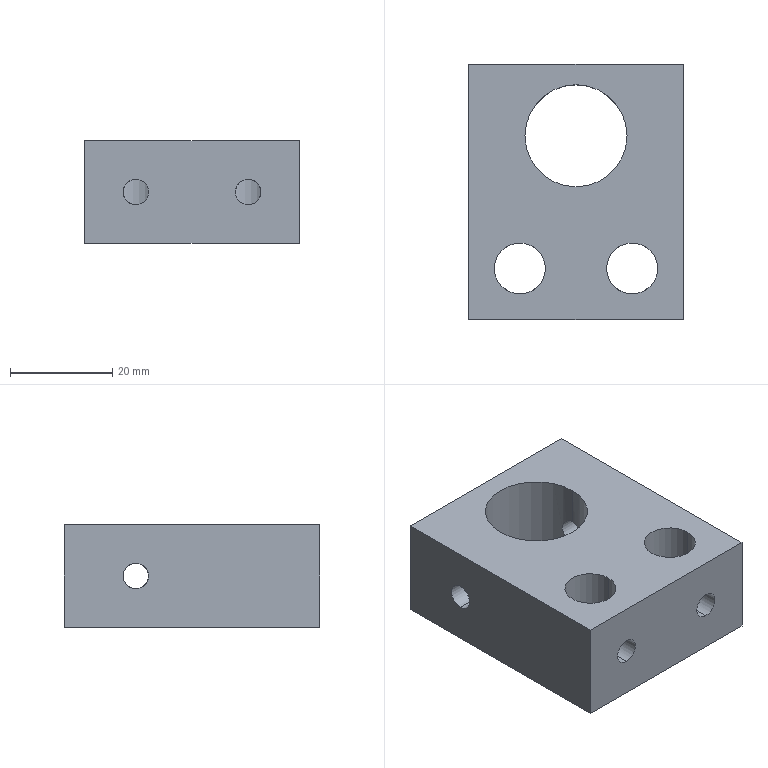Part | STEP file | Switch fixing block 2 | 1 solid | 20 faces | box 42 x 50 x 20 mm | volume 31937 mm3 | cylinder 14 | plane 6 | commonest cylinder face diameters 5 x8 10 x4 20 x2